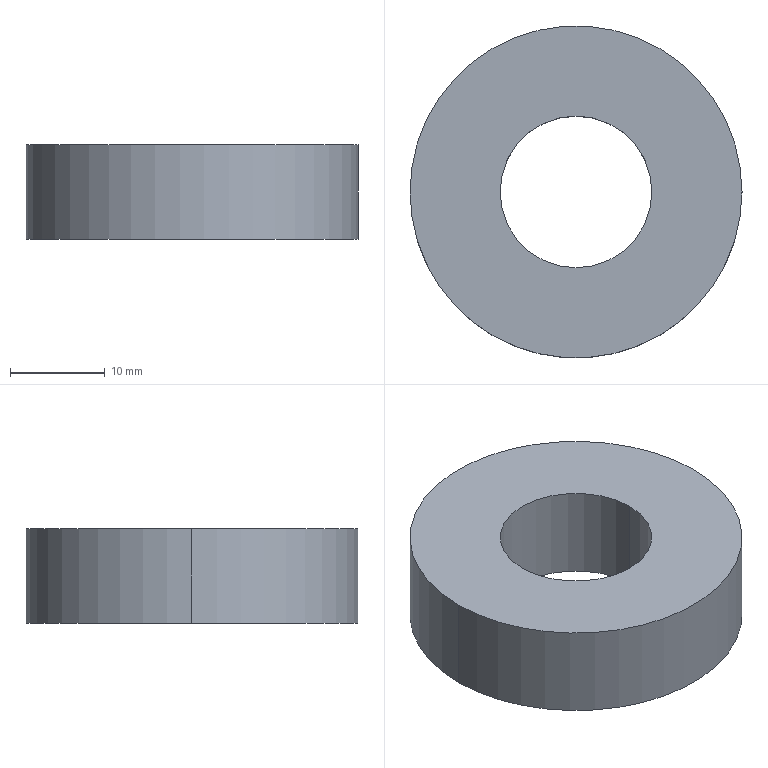Part | STEP file | 1 solid | 6 faces | box 35 x 35 x 10 mm | volume 7611 mm3 | cylinder 4 | plane 2 | commonest cylinder face diameters 16 x2 35 x2
STEP:
#1=CARTESIAN_POINT('',(0.,0.,0.));
#2=DIRECTION('',(0.,0.,1.));
#3=DIRECTION('',(1.,0.,0.));
#4=AXIS2_PLACEMENT_3D('',#1,#2,#3);
#5=CARTESIAN_POINT('',(17.5,0.,-5.));
#6=VERTEX_POINT('',#5);
#7=CARTESIAN_POINT('',(-17.5,0.,-5.));
#8=VERTEX_POINT('',#7);
#9=CARTESIAN_POINT('',(0.,0.,-5.));
#10=DIRECTION('',(0.,0.,-1.));
#11=DIRECTION('',(-1.,0.,0.));
#12=AXIS2_PLACEMENT_3D('',#9,#10,#11);
#13=CIRCLE('',#12,17.5);
#14=CARTESIAN_POINT('',(0.,0.,-5.));
#15=DIRECTION('',(0.,0.,1.));
#16=DIRECTION('',(-1.,0.,0.));
#17=AXIS2_PLACEMENT_3D('',#14,#15,#16);
#18=CYLINDRICAL_SURFACE('',#17,17.5);
#19=CARTESIAN_POINT('',(6.283,0.));
#20=DIRECTION('',(-1.,0.));
#21=VECTOR('',#20,1.);
#22=LINE('',#19,#21);
#23=(GEOMETRIC_REPRESENTATION_CONTEXT(2)PARAMETRIC_REPRESENTATION_CONTEXT()REPRESENTATION_CONTEXT('',''));
#24=DEFINITIONAL_REPRESENTATION('',(#22),#23);
#25=PCURVE('',#18,#24);
#26=CARTESIAN_POINT('',(0.,17.5,-5.));
#27=DIRECTION('',(0.,0.,1.));
#28=DIRECTION('',(1.,0.,0.));
#29=AXIS2_PLACEMENT_3D('',#26,#27,#28);
#30=PLANE('',#29);
#31=CARTESIAN_POINT('',(-17.5,-17.5));
#32=CARTESIAN_POINT('',(-17.5,12.811));
#33=CARTESIAN_POINT('',(8.75,-2.345));
#34=CARTESIAN_POINT('',(35.,-17.5));
#35=CARTESIAN_POINT('',(8.75,-32.655));
#36=CARTESIAN_POINT('',(-17.5,-47.811));
#37=CARTESIAN_POINT('',(-17.5,-17.5));
#38=(BOUNDED_CURVE()B_SPLINE_CURVE(2,(#31,#32,#33,#34,#35,#36,#37),.UNSPECIFIED.,.T.,.F.)B_SPLINE_CURVE_WITH_KNOTS((1,2,2,2,2,1),(-2.094,0.,2.094,4.189,6.283,8.378),.UNSPECIFIED.)CURVE()GEOMETRIC_REPRESENTATION_ITEM()RATIONAL_B_SPLINE_CURVE((1.,0.5,1.,0.5,1.,0.5,1.))REPRESENTATION_ITEM(''));
#39=(GEOMETRIC_REPRESENTATION_CONTEXT(2)PARAMETRIC_REPRESENTATION_CONTEXT()REPRESENTATION_CONTEXT('',''));
#40=DEFINITIONAL_REPRESENTATION('',(#38),#39);
#41=PCURVE('',#30,#40);
#42=SURFACE_CURVE('',#13,(#25,#41),.PCURVE_S1.);
#43=EDGE_CURVE('',#6,#8,#42,.T.);
#44=ORIENTED_EDGE('',*,*,#43,.F.);
#45=CARTESIAN_POINT('',(17.5,0.,5.));
#46=VERTEX_POINT('',#45);
#47=CARTESIAN_POINT('',(17.5,0.,-5.));
#48=DIRECTION('',(0.,0.,1.));
#49=VECTOR('',#48,1.);
#50=LINE('',#47,#49);
#51=CARTESIAN_POINT('',(3.142,0.));
#52=DIRECTION('',(0.,1.));
#53=VECTOR('',#52,1.);
#54=LINE('',#51,#53);
#55=(GEOMETRIC_REPRESENTATION_CONTEXT(2)PARAMETRIC_REPRESENTATION_CONTEXT()REPRESENTATION_CONTEXT('',''));
#56=DEFINITIONAL_REPRESENTATION('',(#54),#55);
#57=PCURVE('',#18,#56);
#58=CARTESIAN_POINT('',(0.,0.,-5.));
#59=DIRECTION('',(0.,0.,1.));
#60=DIRECTION('',(-1.,0.,0.));
#61=AXIS2_PLACEMENT_3D('',#58,#59,#60);
#62=CYLINDRICAL_SURFACE('',#61,17.5);
#63=CARTESIAN_POINT('',(3.142,0.));
#64=DIRECTION('',(0.,1.));
#65=VECTOR('',#64,1.);
#66=LINE('',#63,#65);
#67=(GEOMETRIC_REPRESENTATION_CONTEXT(2)PARAMETRIC_REPRESENTATION_CONTEXT()REPRESENTATION_CONTEXT('',''));
#68=DEFINITIONAL_REPRESENTATION('',(#66),#67);
#69=PCURVE('',#62,#68);
#70=SURFACE_CURVE('',#50,(#57,#69),.PCURVE_S1.);
#71=EDGE_CURVE('',#6,#46,#70,.T.);
#72=ORIENTED_EDGE('',*,*,#71,.T.);
#73=CARTESIAN_POINT('',(-17.5,0.,5.));
#74=VERTEX_POINT('',#73);
#75=CARTESIAN_POINT('',(0.,0.,5.));
#76=DIRECTION('',(0.,0.,-1.));
#77=DIRECTION('',(-1.,0.,0.));
#78=AXIS2_PLACEMENT_3D('',#75,#76,#77);
#79=CIRCLE('',#78,17.5);
#80=CARTESIAN_POINT('',(6.283,10.));
#81=DIRECTION('',(-1.,0.));
#82=VECTOR('',#81,1.);
#83=LINE('',#80,#82);
#84=(GEOMETRIC_REPRESENTATION_CONTEXT(2)PARAMETRIC_REPRESENTATION_CONTEXT()REPRESENTATION_CONTEXT('',''));
#85=DEFINITIONAL_REPRESENTATION('',(#83),#84);
#86=PCURVE('',#18,#85);
#87=CARTESIAN_POINT('',(0.,0.,5.));
#88=DIRECTION('',(0.,0.,-1.));
#89=DIRECTION('',(0.,-1.,0.));
#90=AXIS2_PLACEMENT_3D('',#87,#88,#89);
#91=PLANE('',#90);
#92=CARTESIAN_POINT('',(0.,0.));
#93=DIRECTION('',(0.,1.));
#94=AXIS2_PLACEMENT_2D('',#92,#93);
#95=CIRCLE('',#94,17.5);
#96=(GEOMETRIC_REPRESENTATION_CONTEXT(2)PARAMETRIC_REPRESENTATION_CONTEXT()REPRESENTATION_CONTEXT('',''));
#97=DEFINITIONAL_REPRESENTATION('',(#95),#96);
#98=PCURVE('',#91,#97);
#99=SURFACE_CURVE('',#79,(#86,#98),.PCURVE_S1.);
#100=EDGE_CURVE('',#46,#74,#99,.T.);
#101=ORIENTED_EDGE('',*,*,#100,.T.);
#102=CARTESIAN_POINT('',(-17.5,0.,-5.));
#103=DIRECTION('',(0.,0.,1.));
#104=VECTOR('',#103,1.);
#105=LINE('',#102,#104);
#106=CARTESIAN_POINT('',(0.,0.));
#107=DIRECTION('',(0.,1.));
#108=VECTOR('',#107,1.);
#109=LINE('',#106,#108);
#110=(GEOMETRIC_REPRESENTATION_CONTEXT(2)PARAMETRIC_REPRESENTATION_CONTEXT()REPRESENTATION_CONTEXT('',''));
#111=DEFINITIONAL_REPRESENTATION('',(#109),#110);
#112=PCURVE('',#18,#111);
#113=CARTESIAN_POINT('',(6.283,0.));
#114=DIRECTION('',(0.,1.));
#115=VECTOR('',#114,1.);
#116=LINE('',#113,#115);
#117=(GEOMETRIC_REPRESENTATION_CONTEXT(2)PARAMETRIC_REPRESENTATION_CONTEXT()REPRESENTATION_CONTEXT('',''));
#118=DEFINITIONAL_REPRESENTATION('',(#116),#117);
#119=PCURVE('',#62,#118);
#120=SURFACE_CURVE('',#105,(#112,#119),.PCURVE_S1.);
#121=EDGE_CURVE('',#8,#74,#120,.T.);
#122=ORIENTED_EDGE('',*,*,#121,.F.);
#123=EDGE_LOOP('',(#44,#72,#101,#122));
#124=FACE_BOUND('',#123,.T.);
#125=ADVANCED_FACE('',(#124),#18,.T.);
#126=CARTESIAN_POINT('',(-8.,0.,-5.));
#127=VERTEX_POINT('',#126);
#128=CARTESIAN_POINT('',(-8.,0.,5.));
#129=VERTEX_POINT('',#128);
#130=CARTESIAN_POINT('',(-8.,0.,-5.));
#131=DIRECTION('',(0.,0.,1.));
#132=VECTOR('',#131,1.);
#133=LINE('',#130,#132);
#134=CARTESIAN_POINT('',(0.,0.,-5.));
#135=DIRECTION('',(0.,0.,1.));
#136=DIRECTION('',(-1.,0.,0.));
#137=AXIS2_PLACEMENT_3D('',#134,#135,#136);
#138=CYLINDRICAL_SURFACE('',#137,8.);
#139=CARTESIAN_POINT('',(6.283,0.));
#140=DIRECTION('',(0.,1.));
#141=VECTOR('',#140,1.);
#142=LINE('',#139,#141);
#143=(GEOMETRIC_REPRESENTATION_CONTEXT(2)PARAMETRIC_REPRESENTATION_CONTEXT()REPRESENTATION_CONTEXT('',''));
#144=DEFINITIONAL_REPRESENTATION('',(#142),#143);
#145=PCURVE('',#138,#144);
#146=CARTESIAN_POINT('',(0.,0.,-5.));
#147=DIRECTION('',(0.,0.,1.));
#148=DIRECTION('',(-1.,0.,0.));
#149=AXIS2_PLACEMENT_3D('',#146,#147,#148);
#150=CYLINDRICAL_SURFACE('',#149,8.);
#151=CARTESIAN_POINT('',(0.,0.));
#152=DIRECTION('',(0.,1.));
#153=VECTOR('',#152,1.);
#154=LINE('',#151,#153);
#155=(GEOMETRIC_REPRESENTATION_CONTEXT(2)PARAMETRIC_REPRESENTATION_CONTEXT()REPRESENTATION_CONTEXT('',''));
#156=DEFINITIONAL_REPRESENTATION('',(#154),#155);
#157=PCURVE('',#150,#156);
#158=SURFACE_CURVE('',#133,(#145,#157),.PCURVE_S1.);
#159=EDGE_CURVE('',#127,#129,#158,.T.);
#160=ORIENTED_EDGE('',*,*,#159,.T.);
#161=CARTESIAN_POINT('',(8.,0.,5.));
#162=VERTEX_POINT('',#161);
#163=CARTESIAN_POINT('',(0.,0.,5.));
#164=DIRECTION('',(0.,0.,-1.));
#165=DIRECTION('',(-1.,0.,0.));
#166=AXIS2_PLACEMENT_3D('',#163,#164,#165);
#167=CIRCLE('',#166,8.);
#168=CARTESIAN_POINT('',(6.283,10.));
#169=DIRECTION('',(-1.,0.));
#170=VECTOR('',#169,1.);
#171=LINE('',#168,#170);
#172=(GEOMETRIC_REPRESENTATION_CONTEXT(2)PARAMETRIC_REPRESENTATION_CONTEXT()REPRESENTATION_CONTEXT('',''));
#173=DEFINITIONAL_REPRESENTATION('',(#171),#172);
#174=PCURVE('',#138,#173);
#175=CARTESIAN_POINT('',(0.,0.));
#176=DIRECTION('',(0.,1.));
#177=AXIS2_PLACEMENT_2D('',#175,#176);
#178=CIRCLE('',#177,8.);
#179=(GEOMETRIC_REPRESENTATION_CONTEXT(2)PARAMETRIC_REPRESENTATION_CONTEXT()REPRESENTATION_CONTEXT('',''));
#180=DEFINITIONAL_REPRESENTATION('',(#178),#179);
#181=PCURVE('',#91,#180);
#182=SURFACE_CURVE('',#167,(#174,#181),.PCURVE_S1.);
#183=EDGE_CURVE('',#129,#162,#182,.T.);
#184=ORIENTED_EDGE('',*,*,#183,.T.);
#185=CARTESIAN_POINT('',(8.,0.,-5.));
#186=VERTEX_POINT('',#185);
#187=CARTESIAN_POINT('',(8.,0.,-5.));
#188=DIRECTION('',(0.,0.,1.));
#189=VECTOR('',#188,1.);
#190=LINE('',#187,#189);
#191=CARTESIAN_POINT('',(3.142,0.));
#192=DIRECTION('',(0.,1.));
#193=VECTOR('',#192,1.);
#194=LINE('',#191,#193);
#195=(GEOMETRIC_REPRESENTATION_CONTEXT(2)PARAMETRIC_REPRESENTATION_CONTEXT()REPRESENTATION_CONTEXT('',''));
#196=DEFINITIONAL_REPRESENTATION('',(#194),#195);
#197=PCURVE('',#138,#196);
#198=CARTESIAN_POINT('',(3.142,0.));
#199=DIRECTION('',(0.,1.));
#200=VECTOR('',#199,1.);
#201=LINE('',#198,#200);
#202=(GEOMETRIC_REPRESENTATION_CONTEXT(2)PARAMETRIC_REPRESENTATION_CONTEXT()REPRESENTATION_CONTEXT('',''));
#203=DEFINITIONAL_REPRESENTATION('',(#201),#202);
#204=PCURVE('',#150,#203);
#205=SURFACE_CURVE('',#190,(#197,#204),.PCURVE_S1.);
#206=EDGE_CURVE('',#186,#162,#205,.T.);
#207=ORIENTED_EDGE('',*,*,#206,.F.);
#208=CARTESIAN_POINT('',(0.,0.,-5.));
#209=DIRECTION('',(0.,0.,-1.));
#210=DIRECTION('',(-1.,0.,0.));
#211=AXIS2_PLACEMENT_3D('',#208,#209,#210);
#212=CIRCLE('',#211,8.);
#213=CARTESIAN_POINT('',(6.283,0.));
#214=DIRECTION('',(-1.,0.));
#215=VECTOR('',#214,1.);
#216=LINE('',#213,#215);
#217=(GEOMETRIC_REPRESENTATION_CONTEXT(2)PARAMETRIC_REPRESENTATION_CONTEXT()REPRESENTATION_CONTEXT('',''));
#218=DEFINITIONAL_REPRESENTATION('',(#216),#217);
#219=PCURVE('',#138,#218);
#220=CARTESIAN_POINT('',(-8.,-17.5));
#221=CARTESIAN_POINT('',(-8.,-3.644));
#222=CARTESIAN_POINT('',(4.,-10.572));
#223=CARTESIAN_POINT('',(16.,-17.5));
#224=CARTESIAN_POINT('',(4.,-24.428));
#225=CARTESIAN_POINT('',(-8.,-31.356));
#226=CARTESIAN_POINT('',(-8.,-17.5));
#227=(BOUNDED_CURVE()B_SPLINE_CURVE(2,(#220,#221,#222,#223,#224,#225,#226),.UNSPECIFIED.,.T.,.F.)B_SPLINE_CURVE_WITH_KNOTS((1,2,2,2,2,1),(-2.094,0.,2.094,4.189,6.283,8.378),.UNSPECIFIED.)CURVE()GEOMETRIC_REPRESENTATION_ITEM()RATIONAL_B_SPLINE_CURVE((1.,0.5,1.,0.5,1.,0.5,1.))REPRESENTATION_ITEM(''));
#228=(GEOMETRIC_REPRESENTATION_CONTEXT(2)PARAMETRIC_REPRESENTATION_CONTEXT()REPRESENTATION_CONTEXT('',''));
#229=DEFINITIONAL_REPRESENTATION('',(#227),#228);
#230=PCURVE('',#30,#229);
#231=SURFACE_CURVE('',#212,(#219,#230),.PCURVE_S1.);
#232=EDGE_CURVE('',#127,#186,#231,.T.);
#233=ORIENTED_EDGE('',*,*,#232,.F.);
#234=EDGE_LOOP('',(#160,#184,#207,#233));
#235=FACE_BOUND('',#234,.F.);
#236=ADVANCED_FACE('',(#235),#138,.F.);
#237=CARTESIAN_POINT('',(0.,0.,-5.));
#238=DIRECTION('',(0.,0.,-1.));
#239=DIRECTION('',(-1.,0.,0.));
#240=AXIS2_PLACEMENT_3D('',#237,#238,#239);
#241=CIRCLE('',#240,17.5);
#242=CARTESIAN_POINT('',(-17.5,-17.5));
#243=CARTESIAN_POINT('',(-17.5,12.811));
#244=CARTESIAN_POINT('',(8.75,-2.345));
#245=CARTESIAN_POINT('',(35.,-17.5));
#246=CARTESIAN_POINT('',(8.75,-32.655));
#247=CARTESIAN_POINT('',(-17.5,-47.811));
#248=CARTESIAN_POINT('',(-17.5,-17.5));
#249=(BOUNDED_CURVE()B_SPLINE_CURVE(2,(#242,#243,#244,#245,#246,#247,#248),.UNSPECIFIED.,.T.,.F.)B_SPLINE_CURVE_WITH_KNOTS((1,2,2,2,2,1),(-2.094,0.,2.094,4.189,6.283,8.378),.UNSPECIFIED.)CURVE()GEOMETRIC_REPRESENTATION_ITEM()RATIONAL_B_SPLINE_CURVE((1.,0.5,1.,0.5,1.,0.5,1.))REPRESENTATION_ITEM(''));
#250=(GEOMETRIC_REPRESENTATION_CONTEXT(2)PARAMETRIC_REPRESENTATION_CONTEXT()REPRESENTATION_CONTEXT('',''));
#251=DEFINITIONAL_REPRESENTATION('',(#249),#250);
#252=PCURVE('',#30,#251);
#253=CARTESIAN_POINT('',(6.283,0.));
#254=DIRECTION('',(-1.,0.));
#255=VECTOR('',#254,1.);
#256=LINE('',#253,#255);
#257=(GEOMETRIC_REPRESENTATION_CONTEXT(2)PARAMETRIC_REPRESENTATION_CONTEXT()REPRESENTATION_CONTEXT('',''));
#258=DEFINITIONAL_REPRESENTATION('',(#256),#257);
#259=PCURVE('',#62,#258);
#260=SURFACE_CURVE('',#241,(#252,#259),.PCURVE_S1.);
#261=EDGE_CURVE('',#8,#6,#260,.T.);
#262=ORIENTED_EDGE('',*,*,#261,.T.);
#263=ORIENTED_EDGE('',*,*,#43,.T.);
#264=EDGE_LOOP('',(#262,#263));
#265=FACE_BOUND('',#264,.T.);
#266=ORIENTED_EDGE('',*,*,#232,.F.);
#267=CARTESIAN_POINT('',(0.,0.,-5.));
#268=DIRECTION('',(0.,0.,-1.));
#269=DIRECTION('',(-1.,0.,0.));
#270=AXIS2_PLACEMENT_3D('',#267,#268,#269);
#271=CIRCLE('',#270,8.);
#272=CARTESIAN_POINT('',(-8.,-17.5));
#273=CARTESIAN_POINT('',(-8.,-3.644));
#274=CARTESIAN_POINT('',(4.,-10.572));
#275=CARTESIAN_POINT('',(16.,-17.5));
#276=CARTESIAN_POINT('',(4.,-24.428));
#277=CARTESIAN_POINT('',(-8.,-31.356));
#278=CARTESIAN_POINT('',(-8.,-17.5));
#279=(BOUNDED_CURVE()B_SPLINE_CURVE(2,(#272,#273,#274,#275,#276,#277,#278),.UNSPECIFIED.,.T.,.F.)B_SPLINE_CURVE_WITH_KNOTS((1,2,2,2,2,1),(-2.094,0.,2.094,4.189,6.283,8.378),.UNSPECIFIED.)CURVE()GEOMETRIC_REPRESENTATION_ITEM()RATIONAL_B_SPLINE_CURVE((1.,0.5,1.,0.5,1.,0.5,1.))REPRESENTATION_ITEM(''));
#280=(GEOMETRIC_REPRESENTATION_CONTEXT(2)PARAMETRIC_REPRESENTATION_CONTEXT()REPRESENTATION_CONTEXT('',''));
#281=DEFINITIONAL_REPRESENTATION('',(#279),#280);
#282=PCURVE('',#30,#281);
#283=CARTESIAN_POINT('',(6.283,0.));
#284=DIRECTION('',(-1.,0.));
#285=VECTOR('',#284,1.);
#286=LINE('',#283,#285);
#287=(GEOMETRIC_REPRESENTATION_CONTEXT(2)PARAMETRIC_REPRESENTATION_CONTEXT()REPRESENTATION_CONTEXT('',''));
#288=DEFINITIONAL_REPRESENTATION('',(#286),#287);
#289=PCURVE('',#150,#288);
#290=SURFACE_CURVE('',#271,(#282,#289),.PCURVE_S1.);
#291=EDGE_CURVE('',#186,#127,#290,.T.);
#292=ORIENTED_EDGE('',*,*,#291,.F.);
#293=EDGE_LOOP('',(#266,#292));
#294=FACE_BOUND('',#293,.T.);
#295=ADVANCED_FACE('',(#265,#294),#30,.F.);
#296=CARTESIAN_POINT('',(0.,0.,5.));
#297=DIRECTION('',(0.,0.,-1.));
#298=DIRECTION('',(-1.,0.,0.));
#299=AXIS2_PLACEMENT_3D('',#296,#297,#298);
#300=CIRCLE('',#299,8.);
#301=CARTESIAN_POINT('',(6.283,10.));
#302=DIRECTION('',(-1.,0.));
#303=VECTOR('',#302,1.);
#304=LINE('',#301,#303);
#305=(GEOMETRIC_REPRESENTATION_CONTEXT(2)PARAMETRIC_REPRESENTATION_CONTEXT()REPRESENTATION_CONTEXT('',''));
#306=DEFINITIONAL_REPRESENTATION('',(#304),#305);
#307=PCURVE('',#150,#306);
#308=CARTESIAN_POINT('',(0.,0.));
#309=DIRECTION('',(0.,1.));
#310=AXIS2_PLACEMENT_2D('',#308,#309);
#311=CIRCLE('',#310,8.);
#312=(GEOMETRIC_REPRESENTATION_CONTEXT(2)PARAMETRIC_REPRESENTATION_CONTEXT()REPRESENTATION_CONTEXT('',''));
#313=DEFINITIONAL_REPRESENTATION('',(#311),#312);
#314=PCURVE('',#91,#313);
#315=SURFACE_CURVE('',#300,(#307,#314),.PCURVE_S1.);
#316=EDGE_CURVE('',#162,#129,#315,.T.);
#317=ORIENTED_EDGE('',*,*,#316,.T.);
#318=ORIENTED_EDGE('',*,*,#159,.F.);
#319=ORIENTED_EDGE('',*,*,#291,.F.);
#320=ORIENTED_EDGE('',*,*,#206,.T.);
#321=EDGE_LOOP('',(#317,#318,#319,#320));
#322=FACE_BOUND('',#321,.F.);
#323=ADVANCED_FACE('',(#322),#150,.F.);
#324=ORIENTED_EDGE('',*,*,#71,.F.);
#325=ORIENTED_EDGE('',*,*,#261,.F.);
#326=ORIENTED_EDGE('',*,*,#121,.T.);
#327=CARTESIAN_POINT('',(0.,0.,5.));
#328=DIRECTION('',(0.,0.,-1.));
#329=DIRECTION('',(-1.,0.,0.));
#330=AXIS2_PLACEMENT_3D('',#327,#328,#329);
#331=CIRCLE('',#330,17.5);
#332=CARTESIAN_POINT('',(6.283,10.));
#333=DIRECTION('',(-1.,0.));
#334=VECTOR('',#333,1.);
#335=LINE('',#332,#334);
#336=(GEOMETRIC_REPRESENTATION_CONTEXT(2)PARAMETRIC_REPRESENTATION_CONTEXT()REPRESENTATION_CONTEXT('',''));
#337=DEFINITIONAL_REPRESENTATION('',(#335),#336);
#338=PCURVE('',#62,#337);
#339=CARTESIAN_POINT('',(0.,0.));
#340=DIRECTION('',(0.,1.));
#341=AXIS2_PLACEMENT_2D('',#339,#340);
#342=CIRCLE('',#341,17.5);
#343=(GEOMETRIC_REPRESENTATION_CONTEXT(2)PARAMETRIC_REPRESENTATION_CONTEXT()REPRESENTATION_CONTEXT('',''));
#344=DEFINITIONAL_REPRESENTATION('',(#342),#343);
#345=PCURVE('',#91,#344);
#346=SURFACE_CURVE('',#331,(#338,#345),.PCURVE_S1.);
#347=EDGE_CURVE('',#74,#46,#346,.T.);
#348=ORIENTED_EDGE('',*,*,#347,.T.);
#349=EDGE_LOOP('',(#324,#325,#326,#348));
#350=FACE_BOUND('',#349,.T.);
#351=ADVANCED_FACE('',(#350),#62,.T.);
#352=ORIENTED_EDGE('',*,*,#347,.F.);
#353=ORIENTED_EDGE('',*,*,#100,.F.);
#354=EDGE_LOOP('',(#352,#353));
#355=FACE_BOUND('',#354,.T.);
#356=ORIENTED_EDGE('',*,*,#183,.T.);
#357=ORIENTED_EDGE('',*,*,#316,.T.);
#358=EDGE_LOOP('',(#356,#357));
#359=FACE_BOUND('',#358,.T.);
#360=ADVANCED_FACE('',(#355,#359),#91,.F.);
#361=CLOSED_SHELL('',(#125,#236,#295,#323,#351,#360));
#362=MANIFOLD_SOLID_BREP('',#361);
#363=(LENGTH_UNIT()NAMED_UNIT(*)SI_UNIT(.MILLI.,.METRE.));
#364=UNCERTAINTY_MEASURE_WITH_UNIT(LENGTH_MEASURE(0.0000001),#363,'','');
#365=(NAMED_UNIT(*)PLANE_ANGLE_UNIT()SI_UNIT($,.RADIAN.));
#366=(NAMED_UNIT(*)SI_UNIT($,.STERADIAN.)SOLID_ANGLE_UNIT());
#367=(GEOMETRIC_REPRESENTATION_CONTEXT(3)GLOBAL_UNCERTAINTY_ASSIGNED_CONTEXT((#364))GLOBAL_UNIT_ASSIGNED_CONTEXT((#363,#365,#366))REPRESENTATION_CONTEXT('',''));
#368=ADVANCED_BREP_SHAPE_REPRESENTATION('',(#4,#362),#367);